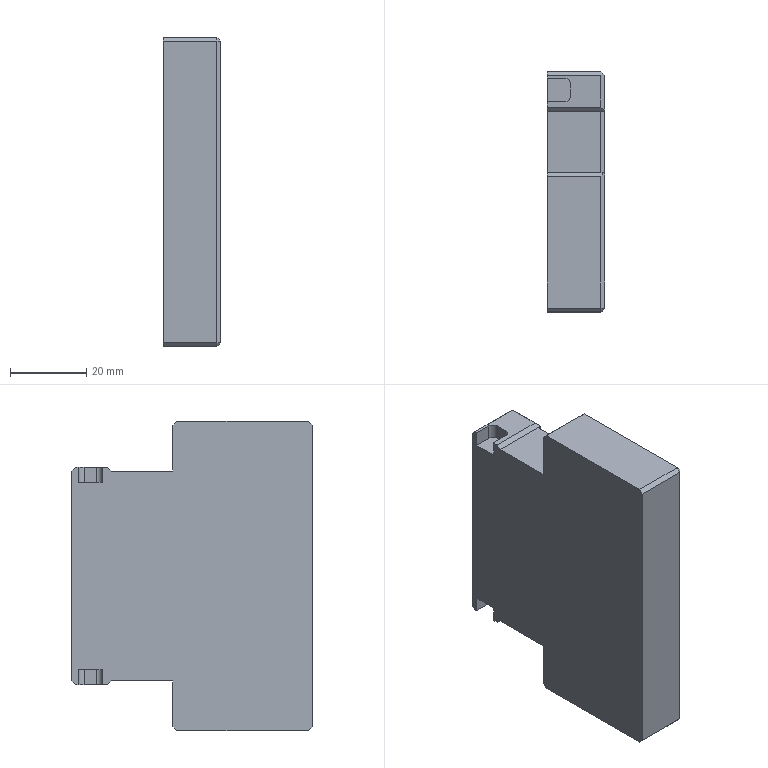Part | STEP file | 1 solid | 110 faces | box 15 x 63 x 81 mm | volume 65609 mm3 | plane 82 | cylinder 20 | spline 8 | commonest cylinder face diameters 7 x8 8 x8 3 x4